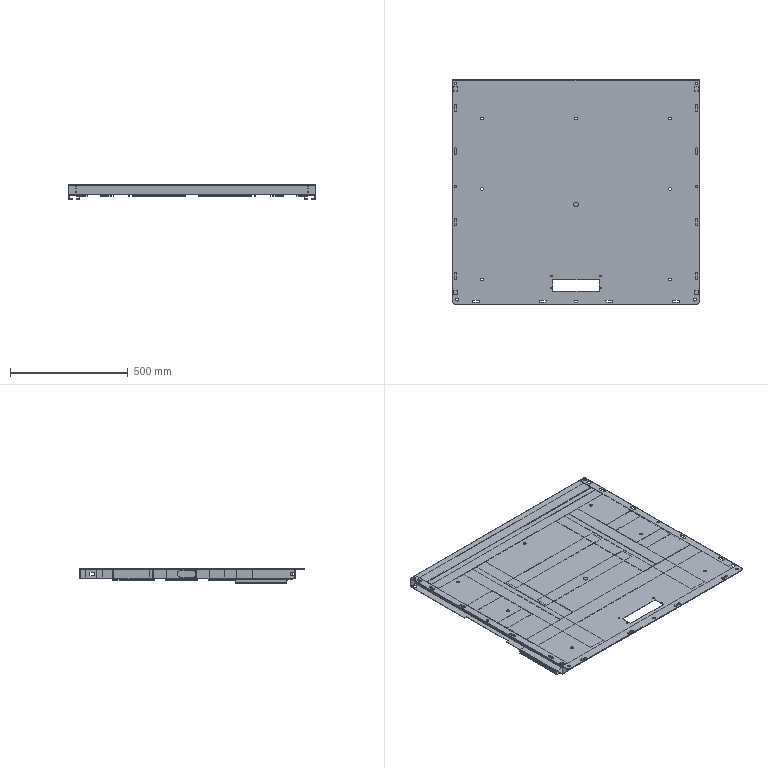Part | 27 solids | 1678 faces | box 1050 x 955 x 63.5 mm | volume 4316742 mm3 | plane 1211 | cylinder 443 | cone 24 | commonest cylinder face diameters 0.4 x102 3.4 x100 10 x84 20 x38 6 x20 11 x17